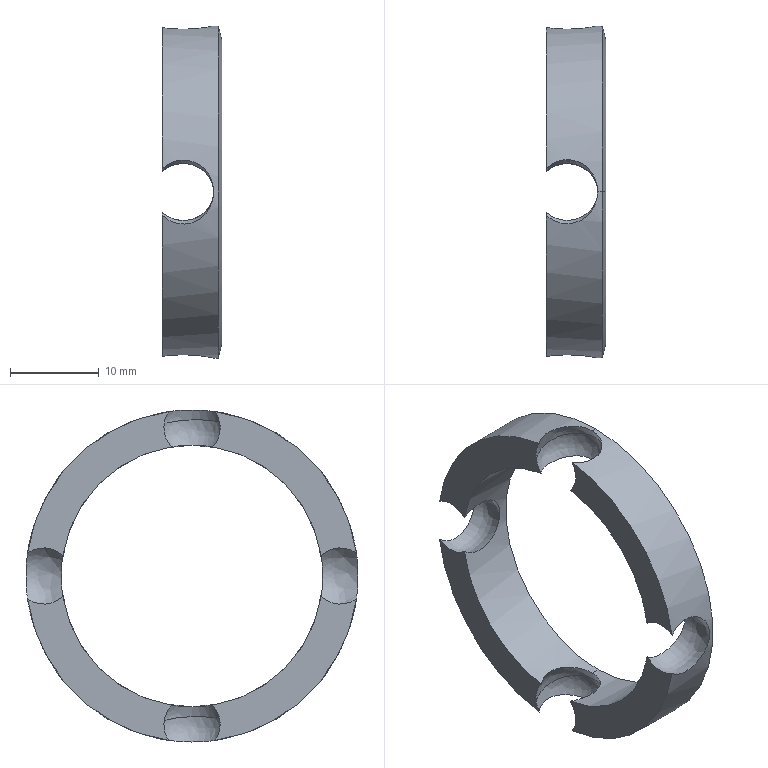Part | STEP file | Microwave Drying Flat Conveyor-inafag_ucfl204_62o9y6gnj3059x015y4y3bh4_14 | 1 solid | 17 faces | volume 2155 mm3 | spline 6 | plane 5 | cylinder 4 | cone 2 | commonest cylinder face diameters 29.53 x2 37.47 x2